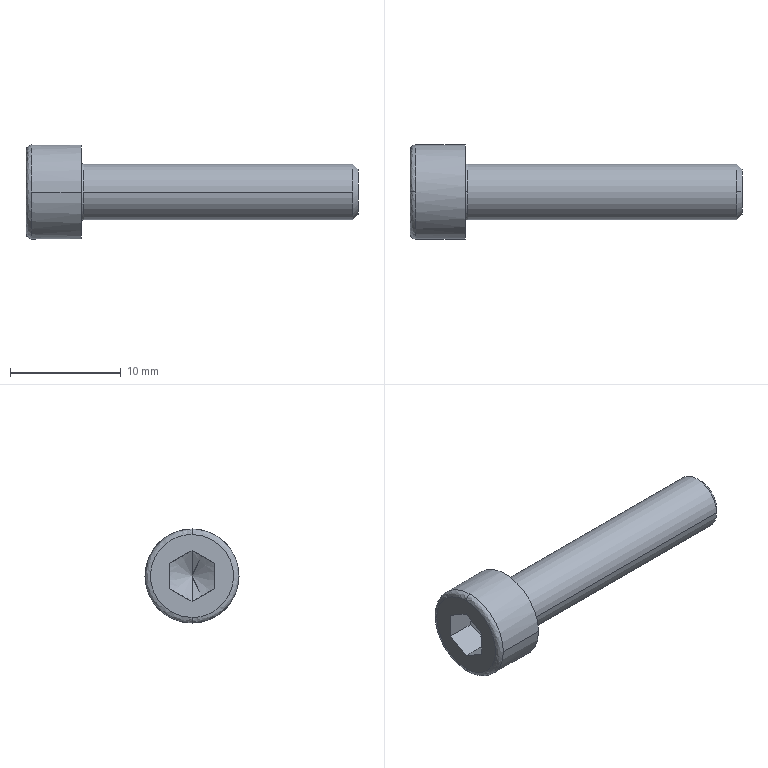Part | STEP file | Broached Socket Head Cap Screw - Metric M5x0.8 x 25 | 1 solid | 21 faces | box 30 x 8.5 x 8.5 mm | volume 729.698 mm3 | plane 9 | spline 4 | cylinder 4 | cone 4 | commonest cylinder face diameters 5 x2 8.5 x2